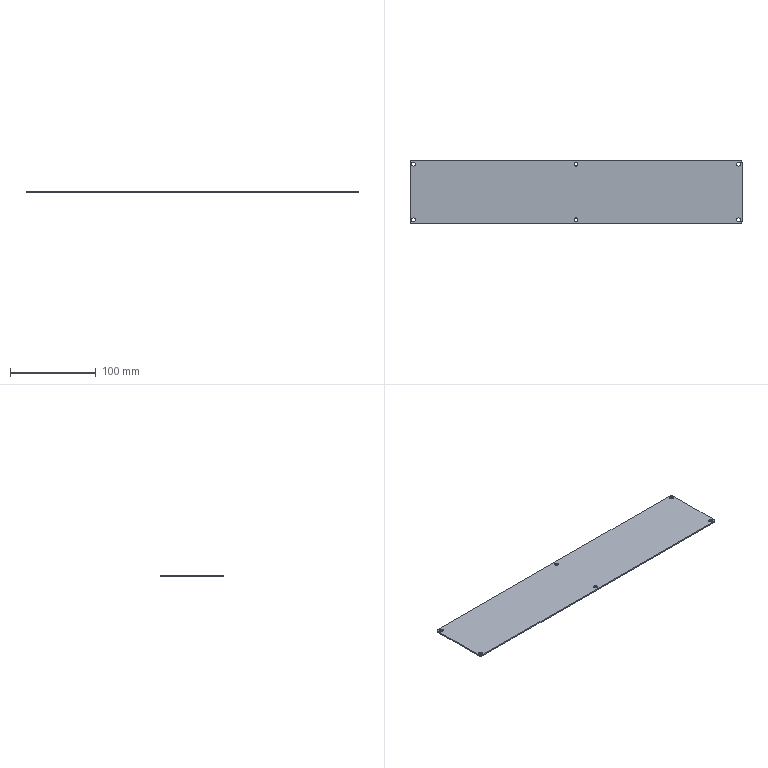Part | NX | features solid 2 | 1 solid | 22 faces | box 388 x 73 x 1.5 mm | volume 42338 mm3 | cylinder 16 | plane 6 | commonest cylinder face diameters 4.5 x12 4 x4
STEP:
#1=CARTESIAN_POINT('',(-842.,-1596.,1025.));
#2=VERTEX_POINT('',#1);
#3=CARTESIAN_POINT('',(-844.,-1598.,1025.));
#4=VERTEX_POINT('',#3);
#5=CARTESIAN_POINT('',(-842.,-1598.,1025.));
#6=DIRECTION('',(0.,0.,1.));
#7=DIRECTION('',(1.,0.,0.));
#8=AXIS2_PLACEMENT_3D('',#5,#6,#7);
#9=CIRCLE('',#8,2.);
#10=EDGE_CURVE('',#2,#4,#9,.T.);
#11=ORIENTED_EDGE('',*,*,#10,.F.);
#12=CARTESIAN_POINT('',(-842.,-1596.,1023.5));
#13=VERTEX_POINT('',#12);
#14=CARTESIAN_POINT('',(-842.,-1596.,1025.));
#15=DIRECTION('',(0.,0.,1.));
#16=VECTOR('',#15,1000.);
#17=LINE('',#14,#16);
#18=EDGE_CURVE('',#13,#2,#17,.T.);
#19=ORIENTED_EDGE('',*,*,#18,.F.);
#20=CARTESIAN_POINT('',(-844.,-1598.,1023.5));
#21=VERTEX_POINT('',#20);
#22=CARTESIAN_POINT('',(-842.,-1598.,1023.5));
#23=DIRECTION('',(0.,0.,-1.));
#24=DIRECTION('',(1.,0.,0.));
#25=AXIS2_PLACEMENT_3D('',#22,#23,#24);
#26=CIRCLE('',#25,2.);
#27=EDGE_CURVE('',#21,#13,#26,.T.);
#28=ORIENTED_EDGE('',*,*,#27,.F.);
#29=CARTESIAN_POINT('',(-844.,-1598.,1025.));
#30=DIRECTION('',(0.,0.,-1.));
#31=VECTOR('',#30,1000.);
#32=LINE('',#29,#31);
#33=EDGE_CURVE('',#4,#21,#32,.T.);
#34=ORIENTED_EDGE('',*,*,#33,.F.);
#35=EDGE_LOOP('',(#11,#19,#28,#34));
#36=FACE_BOUND('',#35,.T.);
#37=CARTESIAN_POINT('',(-842.,-1598.,1025.));
#38=DIRECTION('',(0.,0.,-1.));
#39=DIRECTION('',(-1.,0.,0.));
#40=AXIS2_PLACEMENT_3D('',#37,#38,#39);
#41=CYLINDRICAL_SURFACE('',#40,2.);
#42=ADVANCED_FACE('',(#36),#41,.T.);
#43=CARTESIAN_POINT('',(-844.,-1667.,1025.));
#44=VERTEX_POINT('',#43);
#45=CARTESIAN_POINT('',(-842.,-1669.,1025.));
#46=VERTEX_POINT('',#45);
#47=CARTESIAN_POINT('',(-842.,-1667.,1025.));
#48=DIRECTION('',(0.,0.,1.));
#49=DIRECTION('',(1.,0.,0.));
#50=AXIS2_PLACEMENT_3D('',#47,#48,#49);
#51=CIRCLE('',#50,2.);
#52=EDGE_CURVE('',#44,#46,#51,.T.);
#53=ORIENTED_EDGE('',*,*,#52,.F.);
#54=CARTESIAN_POINT('',(-844.,-1667.,1023.5));
#55=VERTEX_POINT('',#54);
#56=CARTESIAN_POINT('',(-844.,-1667.,1025.));
#57=DIRECTION('',(0.,0.,1.));
#58=VECTOR('',#57,1000.);
#59=LINE('',#56,#58);
#60=EDGE_CURVE('',#55,#44,#59,.T.);
#61=ORIENTED_EDGE('',*,*,#60,.F.);
#62=CARTESIAN_POINT('',(-842.,-1669.,1023.5));
#63=VERTEX_POINT('',#62);
#64=CARTESIAN_POINT('',(-842.,-1667.,1023.5));
#65=DIRECTION('',(0.,0.,-1.));
#66=DIRECTION('',(1.,0.,0.));
#67=AXIS2_PLACEMENT_3D('',#64,#65,#66);
#68=CIRCLE('',#67,2.);
#69=EDGE_CURVE('',#63,#55,#68,.T.);
#70=ORIENTED_EDGE('',*,*,#69,.F.);
#71=CARTESIAN_POINT('',(-842.,-1669.,1025.));
#72=DIRECTION('',(0.,0.,-1.));
#73=VECTOR('',#72,1000.);
#74=LINE('',#71,#73);
#75=EDGE_CURVE('',#46,#63,#74,.T.);
#76=ORIENTED_EDGE('',*,*,#75,.F.);
#77=EDGE_LOOP('',(#53,#61,#70,#76));
#78=FACE_BOUND('',#77,.T.);
#79=CARTESIAN_POINT('',(-842.,-1667.,1025.));
#80=DIRECTION('',(0.,0.,-1.));
#81=DIRECTION('',(-1.,0.,0.));
#82=AXIS2_PLACEMENT_3D('',#79,#80,#81);
#83=CYLINDRICAL_SURFACE('',#82,2.);
#84=ADVANCED_FACE('',(#78),#83,.T.);
#85=CARTESIAN_POINT('',(-458.,-1669.,1025.));
#86=VERTEX_POINT('',#85);
#87=CARTESIAN_POINT('',(-456.,-1667.,1025.));
#88=VERTEX_POINT('',#87);
#89=CARTESIAN_POINT('',(-458.,-1667.,1025.));
#90=DIRECTION('',(0.,0.,1.));
#91=DIRECTION('',(1.,0.,0.));
#92=AXIS2_PLACEMENT_3D('',#89,#90,#91);
#93=CIRCLE('',#92,2.);
#94=EDGE_CURVE('',#86,#88,#93,.T.);
#95=ORIENTED_EDGE('',*,*,#94,.F.);
#96=CARTESIAN_POINT('',(-458.,-1669.,1023.5));
#97=VERTEX_POINT('',#96);
#98=CARTESIAN_POINT('',(-458.,-1669.,1025.));
#99=DIRECTION('',(0.,0.,1.));
#100=VECTOR('',#99,1000.);
#101=LINE('',#98,#100);
#102=EDGE_CURVE('',#97,#86,#101,.T.);
#103=ORIENTED_EDGE('',*,*,#102,.F.);
#104=CARTESIAN_POINT('',(-456.,-1667.,1023.5));
#105=VERTEX_POINT('',#104);
#106=CARTESIAN_POINT('',(-458.,-1667.,1023.5));
#107=DIRECTION('',(0.,0.,-1.));
#108=DIRECTION('',(1.,0.,0.));
#109=AXIS2_PLACEMENT_3D('',#106,#107,#108);
#110=CIRCLE('',#109,2.);
#111=EDGE_CURVE('',#105,#97,#110,.T.);
#112=ORIENTED_EDGE('',*,*,#111,.F.);
#113=CARTESIAN_POINT('',(-456.,-1667.,1025.));
#114=DIRECTION('',(0.,0.,-1.));
#115=VECTOR('',#114,1000.);
#116=LINE('',#113,#115);
#117=EDGE_CURVE('',#88,#105,#116,.T.);
#118=ORIENTED_EDGE('',*,*,#117,.F.);
#119=EDGE_LOOP('',(#95,#103,#112,#118));
#120=FACE_BOUND('',#119,.T.);
#121=CARTESIAN_POINT('',(-458.,-1667.,1025.));
#122=DIRECTION('',(0.,0.,-1.));
#123=DIRECTION('',(-1.,0.,0.));
#124=AXIS2_PLACEMENT_3D('',#121,#122,#123);
#125=CYLINDRICAL_SURFACE('',#124,2.);
#126=ADVANCED_FACE('',(#120),#125,.T.);
#127=CARTESIAN_POINT('',(-456.,-1598.,1025.));
#128=VERTEX_POINT('',#127);
#129=CARTESIAN_POINT('',(-458.,-1596.,1025.));
#130=VERTEX_POINT('',#129);
#131=CARTESIAN_POINT('',(-458.,-1598.,1025.));
#132=DIRECTION('',(0.,0.,1.));
#133=DIRECTION('',(1.,0.,0.));
#134=AXIS2_PLACEMENT_3D('',#131,#132,#133);
#135=CIRCLE('',#134,2.);
#136=EDGE_CURVE('',#128,#130,#135,.T.);
#137=ORIENTED_EDGE('',*,*,#136,.F.);
#138=CARTESIAN_POINT('',(-456.,-1598.,1023.5));
#139=VERTEX_POINT('',#138);
#140=CARTESIAN_POINT('',(-456.,-1598.,1025.));
#141=DIRECTION('',(0.,0.,1.));
#142=VECTOR('',#141,1000.);
#143=LINE('',#140,#142);
#144=EDGE_CURVE('',#139,#128,#143,.T.);
#145=ORIENTED_EDGE('',*,*,#144,.F.);
#146=CARTESIAN_POINT('',(-458.,-1596.,1023.5));
#147=VERTEX_POINT('',#146);
#148=CARTESIAN_POINT('',(-458.,-1598.,1023.5));
#149=DIRECTION('',(0.,0.,-1.));
#150=DIRECTION('',(1.,0.,0.));
#151=AXIS2_PLACEMENT_3D('',#148,#149,#150);
#152=CIRCLE('',#151,2.);
#153=EDGE_CURVE('',#147,#139,#152,.T.);
#154=ORIENTED_EDGE('',*,*,#153,.F.);
#155=CARTESIAN_POINT('',(-458.,-1596.,1025.));
#156=DIRECTION('',(0.,0.,-1.));
#157=VECTOR('',#156,1000.);
#158=LINE('',#155,#157);
#159=EDGE_CURVE('',#130,#147,#158,.T.);
#160=ORIENTED_EDGE('',*,*,#159,.F.);
#161=EDGE_LOOP('',(#137,#145,#154,#160));
#162=FACE_BOUND('',#161,.T.);
#163=CARTESIAN_POINT('',(-458.,-1598.,1025.));
#164=DIRECTION('',(0.,0.,-1.));
#165=DIRECTION('',(-1.,0.,0.));
#166=AXIS2_PLACEMENT_3D('',#163,#164,#165);
#167=CYLINDRICAL_SURFACE('',#166,2.);
#168=ADVANCED_FACE('',(#162),#167,.T.);
#169=CARTESIAN_POINT('',(-652.25,-1600.,1025.));
#170=VERTEX_POINT('',#169);
#171=CARTESIAN_POINT('',(-652.25,-1600.,1023.5));
#172=VERTEX_POINT('',#171);
#173=CARTESIAN_POINT('',(-652.25,-1600.,630.19));
#174=DIRECTION('',(0.,0.,1.));
#175=VECTOR('',#174,1000.);
#176=LINE('',#173,#175);
#177=EDGE_CURVE('',#170,#172,#176,.F.);
#178=ORIENTED_EDGE('',*,*,#177,.T.);
#179=CARTESIAN_POINT('',(-647.75,-1600.,1023.5));
#180=VERTEX_POINT('',#179);
#181=CARTESIAN_POINT('',(-650.,-1600.,1023.5));
#182=DIRECTION('',(0.,0.,1.));
#183=DIRECTION('',(1.,0.,0.));
#184=AXIS2_PLACEMENT_3D('',#181,#182,#183);
#185=CIRCLE('',#184,2.25);
#186=EDGE_CURVE('',#180,#172,#185,.T.);
#187=ORIENTED_EDGE('',*,*,#186,.F.);
#188=CARTESIAN_POINT('',(-647.75,-1600.,1025.));
#189=VERTEX_POINT('',#188);
#190=CARTESIAN_POINT('',(-647.75,-1600.,630.19));
#191=DIRECTION('',(0.,0.,1.));
#192=VECTOR('',#191,1000.);
#193=LINE('',#190,#192);
#194=EDGE_CURVE('',#180,#189,#193,.T.);
#195=ORIENTED_EDGE('',*,*,#194,.T.);
#196=CARTESIAN_POINT('',(-650.,-1600.,1025.));
#197=DIRECTION('',(0.,0.,1.));
#198=DIRECTION('',(0.,1.,0.));
#199=AXIS2_PLACEMENT_3D('',#196,#197,#198);
#200=CIRCLE('',#199,2.25);
#201=EDGE_CURVE('',#189,#170,#200,.T.);
#202=ORIENTED_EDGE('',*,*,#201,.T.);
#203=EDGE_LOOP('',(#178,#187,#195,#202));
#204=FACE_BOUND('',#203,.T.);
#205=CARTESIAN_POINT('',(-650.,-1600.,630.19));
#206=DIRECTION('',(0.,0.,1.));
#207=DIRECTION('',(1.,0.,0.));
#208=AXIS2_PLACEMENT_3D('',#205,#206,#207);
#209=CYLINDRICAL_SURFACE('',#208,2.25);
#210=ADVANCED_FACE('',(#204),#209,.F.);
#211=CARTESIAN_POINT('',(-652.25,-1665.,1023.5));
#212=VERTEX_POINT('',#211);
#213=CARTESIAN_POINT('',(-652.25,-1665.,1025.));
#214=VERTEX_POINT('',#213);
#215=CARTESIAN_POINT('',(-652.25,-1665.,630.19));
#216=DIRECTION('',(0.,0.,1.));
#217=VECTOR('',#216,1000.);
#218=LINE('',#215,#217);
#219=EDGE_CURVE('',#212,#214,#218,.T.);
#220=ORIENTED_EDGE('',*,*,#219,.F.);
#221=CARTESIAN_POINT('',(-647.75,-1665.,1023.5));
#222=VERTEX_POINT('',#221);
#223=CARTESIAN_POINT('',(-650.,-1665.,1023.5));
#224=DIRECTION('',(0.,0.,1.));
#225=DIRECTION('',(1.,0.,0.));
#226=AXIS2_PLACEMENT_3D('',#223,#224,#225);
#227=CIRCLE('',#226,2.25);
#228=EDGE_CURVE('',#222,#212,#227,.T.);
#229=ORIENTED_EDGE('',*,*,#228,.F.);
#230=CARTESIAN_POINT('',(-647.75,-1665.,1025.));
#231=VERTEX_POINT('',#230);
#232=CARTESIAN_POINT('',(-647.75,-1665.,630.19));
#233=DIRECTION('',(0.,0.,1.));
#234=VECTOR('',#233,1000.);
#235=LINE('',#232,#234);
#236=EDGE_CURVE('',#231,#222,#235,.F.);
#237=ORIENTED_EDGE('',*,*,#236,.F.);
#238=CARTESIAN_POINT('',(-650.,-1665.,1025.));
#239=DIRECTION('',(0.,0.,1.));
#240=DIRECTION('',(0.,1.,0.));
#241=AXIS2_PLACEMENT_3D('',#238,#239,#240);
#242=CIRCLE('',#241,2.25);
#243=EDGE_CURVE('',#231,#214,#242,.T.);
#244=ORIENTED_EDGE('',*,*,#243,.T.);
#245=EDGE_LOOP('',(#220,#229,#237,#244));
#246=FACE_BOUND('',#245,.T.);
#247=CARTESIAN_POINT('',(-650.,-1665.,630.19));
#248=DIRECTION('',(0.,0.,1.));
#249=DIRECTION('',(1.,0.,0.));
#250=AXIS2_PLACEMENT_3D('',#247,#248,#249);
#251=CYLINDRICAL_SURFACE('',#250,2.25);
#252=ADVANCED_FACE('',(#246),#251,.F.);
#253=CARTESIAN_POINT('',(-842.25,-1600.,1025.));
#254=VERTEX_POINT('',#253);
#255=CARTESIAN_POINT('',(-842.25,-1600.,1023.5));
#256=VERTEX_POINT('',#255);
#257=CARTESIAN_POINT('',(-842.25,-1600.,630.19));
#258=DIRECTION('',(0.,0.,1.));
#259=VECTOR('',#258,1000.);
#260=LINE('',#257,#259);
#261=EDGE_CURVE('',#254,#256,#260,.F.);
#262=ORIENTED_EDGE('',*,*,#261,.T.);
#263=CARTESIAN_POINT('',(-837.75,-1600.,1023.5));
#264=VERTEX_POINT('',#263);
#265=CARTESIAN_POINT('',(-840.,-1600.,1023.5));
#266=DIRECTION('',(0.,0.,1.));
#267=DIRECTION('',(1.,0.,0.));
#268=AXIS2_PLACEMENT_3D('',#265,#266,#267);
#269=CIRCLE('',#268,2.25);
#270=EDGE_CURVE('',#264,#256,#269,.T.);
#271=ORIENTED_EDGE('',*,*,#270,.F.);
#272=CARTESIAN_POINT('',(-837.75,-1600.,1025.));
#273=VERTEX_POINT('',#272);
#274=CARTESIAN_POINT('',(-837.75,-1600.,630.19));
#275=DIRECTION('',(0.,0.,1.));
#276=VECTOR('',#275,1000.);
#277=LINE('',#274,#276);
#278=EDGE_CURVE('',#264,#273,#277,.T.);
#279=ORIENTED_EDGE('',*,*,#278,.T.);
#280=CARTESIAN_POINT('',(-840.,-1600.,1025.));
#281=DIRECTION('',(0.,0.,1.));
#282=DIRECTION('',(0.,1.,0.));
#283=AXIS2_PLACEMENT_3D('',#280,#281,#282);
#284=CIRCLE('',#283,2.25);
#285=EDGE_CURVE('',#273,#254,#284,.T.);
#286=ORIENTED_EDGE('',*,*,#285,.T.);
#287=EDGE_LOOP('',(#262,#271,#279,#286));
#288=FACE_BOUND('',#287,.T.);
#289=CARTESIAN_POINT('',(-840.,-1600.,630.19));
#290=DIRECTION('',(0.,0.,1.));
#291=DIRECTION('',(1.,0.,0.));
#292=AXIS2_PLACEMENT_3D('',#289,#290,#291);
#293=CYLINDRICAL_SURFACE('',#292,2.25);
#294=ADVANCED_FACE('',(#288),#293,.F.);
#295=CARTESIAN_POINT('',(-462.25,-1600.,1025.));
#296=VERTEX_POINT('',#295);
#297=CARTESIAN_POINT('',(-462.25,-1600.,1023.5));
#298=VERTEX_POINT('',#297);
#299=CARTESIAN_POINT('',(-462.25,-1600.,630.19));
#300=DIRECTION('',(0.,0.,1.));
#301=VECTOR('',#300,1000.);
#302=LINE('',#299,#301);
#303=EDGE_CURVE('',#296,#298,#302,.F.);
#304=ORIENTED_EDGE('',*,*,#303,.T.);
#305=CARTESIAN_POINT('',(-457.75,-1600.,1023.5));
#306=VERTEX_POINT('',#305);
#307=CARTESIAN_POINT('',(-460.,-1600.,1023.5));
#308=DIRECTION('',(0.,0.,1.));
#309=DIRECTION('',(1.,0.,0.));
#310=AXIS2_PLACEMENT_3D('',#307,#308,#309);
#311=CIRCLE('',#310,2.25);
#312=EDGE_CURVE('',#306,#298,#311,.T.);
#313=ORIENTED_EDGE('',*,*,#312,.F.);
#314=CARTESIAN_POINT('',(-457.75,-1600.,1025.));
#315=VERTEX_POINT('',#314);
#316=CARTESIAN_POINT('',(-457.75,-1600.,630.19));
#317=DIRECTION('',(0.,0.,1.));
#318=VECTOR('',#317,1000.);
#319=LINE('',#316,#318);
#320=EDGE_CURVE('',#306,#315,#319,.T.);
#321=ORIENTED_EDGE('',*,*,#320,.T.);
#322=CARTESIAN_POINT('',(-460.,-1600.,1025.));
#323=DIRECTION('',(0.,0.,1.));
#324=DIRECTION('',(0.,1.,0.));
#325=AXIS2_PLACEMENT_3D('',#322,#323,#324);
#326=CIRCLE('',#325,2.25);
#327=EDGE_CURVE('',#315,#296,#326,.T.);
#328=ORIENTED_EDGE('',*,*,#327,.T.);
#329=EDGE_LOOP('',(#304,#313,#321,#328));
#330=FACE_BOUND('',#329,.T.);
#331=CARTESIAN_POINT('',(-460.,-1600.,630.19));
#332=DIRECTION('',(0.,0.,1.));
#333=DIRECTION('',(1.,0.,0.));
#334=AXIS2_PLACEMENT_3D('',#331,#332,#333);
#335=CYLINDRICAL_SURFACE('',#334,2.25);
#336=ADVANCED_FACE('',(#330),#335,.F.);
#337=CARTESIAN_POINT('',(-462.25,-1665.,1023.5));
#338=VERTEX_POINT('',#337);
#339=CARTESIAN_POINT('',(-462.25,-1665.,1025.));
#340=VERTEX_POINT('',#339);
#341=CARTESIAN_POINT('',(-462.25,-1665.,630.19));
#342=DIRECTION('',(0.,0.,1.));
#343=VECTOR('',#342,1000.);
#344=LINE('',#341,#343);
#345=EDGE_CURVE('',#338,#340,#344,.T.);
#346=ORIENTED_EDGE('',*,*,#345,.F.);
#347=CARTESIAN_POINT('',(-457.75,-1665.,1023.5));
#348=VERTEX_POINT('',#347);
#349=CARTESIAN_POINT('',(-460.,-1665.,1023.5));
#350=DIRECTION('',(0.,0.,1.));
#351=DIRECTION('',(1.,0.,0.));
#352=AXIS2_PLACEMENT_3D('',#349,#350,#351);
#353=CIRCLE('',#352,2.25);
#354=EDGE_CURVE('',#348,#338,#353,.T.);
#355=ORIENTED_EDGE('',*,*,#354,.F.);
#356=CARTESIAN_POINT('',(-457.75,-1665.,1025.));
#357=VERTEX_POINT('',#356);
#358=CARTESIAN_POINT('',(-457.75,-1665.,630.19));
#359=DIRECTION('',(0.,0.,1.));
#360=VECTOR('',#359,1000.);
#361=LINE('',#358,#360);
#362=EDGE_CURVE('',#357,#348,#361,.F.);
#363=ORIENTED_EDGE('',*,*,#362,.F.);
#364=CARTESIAN_POINT('',(-460.,-1665.,1025.));
#365=DIRECTION('',(0.,0.,1.));
#366=DIRECTION('',(0.,1.,0.));
#367=AXIS2_PLACEMENT_3D('',#364,#365,#366);
#368=CIRCLE('',#367,2.25);
#369=EDGE_CURVE('',#357,#340,#368,.T.);
#370=ORIENTED_EDGE('',*,*,#369,.T.);
#371=EDGE_LOOP('',(#346,#355,#363,#370));
#372=FACE_BOUND('',#371,.T.);
#373=CARTESIAN_POINT('',(-460.,-1665.,630.19));
#374=DIRECTION('',(0.,0.,1.));
#375=DIRECTION('',(1.,0.,0.));
#376=AXIS2_PLACEMENT_3D('',#373,#374,#375);
#377=CYLINDRICAL_SURFACE('',#376,2.25);
#378=ADVANCED_FACE('',(#372),#377,.F.);
#379=CARTESIAN_POINT('',(-842.25,-1665.,1025.));
#380=VERTEX_POINT('',#379);
#381=CARTESIAN_POINT('',(-842.25,-1665.,1023.5));
#382=VERTEX_POINT('',#381);
#383=CARTESIAN_POINT('',(-842.25,-1665.,630.19));
#384=DIRECTION('',(0.,0.,1.));
#385=VECTOR('',#384,1000.);
#386=LINE('',#383,#385);
#387=EDGE_CURVE('',#380,#382,#386,.F.);
#388=ORIENTED_EDGE('',*,*,#387,.T.);
#389=CARTESIAN_POINT('',(-837.75,-1665.,1023.5));
#390=VERTEX_POINT('',#389);
#391=CARTESIAN_POINT('',(-840.,-1665.,1023.5));
#392=DIRECTION('',(0.,0.,1.));
#393=DIRECTION('',(1.,0.,0.));
#394=AXIS2_PLACEMENT_3D('',#391,#392,#393);
#395=CIRCLE('',#394,2.25);
#396=EDGE_CURVE('',#390,#382,#395,.T.);
#397=ORIENTED_EDGE('',*,*,#396,.F.);
#398=CARTESIAN_POINT('',(-837.75,-1665.,1025.));
#399=VERTEX_POINT('',#398);
#400=CARTESIAN_POINT('',(-837.75,-1665.,630.19));
#401=DIRECTION('',(0.,0.,1.));
#402=VECTOR('',#401,1000.);
#403=LINE('',#400,#402);
#404=EDGE_CURVE('',#390,#399,#403,.T.);
#405=ORIENTED_EDGE('',*,*,#404,.T.);
#406=CARTESIAN_POINT('',(-840.,-1665.,1025.));
#407=DIRECTION('',(0.,0.,1.));
#408=DIRECTION('',(0.,1.,0.));
#409=AXIS2_PLACEMENT_3D('',#406,#407,#408);
#410=CIRCLE('',#409,2.25);
#411=EDGE_CURVE('',#399,#380,#410,.T.);
#412=ORIENTED_EDGE('',*,*,#411,.T.);
#413=EDGE_LOOP('',(#388,#397,#405,#412));
#414=FACE_BOUND('',#413,.T.);
#415=CARTESIAN_POINT('',(-840.,-1665.,630.19));
#416=DIRECTION('',(0.,0.,1.));
#417=DIRECTION('',(1.,0.,0.));
#418=AXIS2_PLACEMENT_3D('',#415,#416,#417);
#419=CYLINDRICAL_SURFACE('',#418,2.25);
#420=ADVANCED_FACE('',(#414),#419,.F.);
#421=ORIENTED_EDGE('',*,*,#396,.T.);
#422=CARTESIAN_POINT('',(-840.,-1665.,1023.5));
#423=DIRECTION('',(0.,0.,1.));
#424=DIRECTION('',(1.,0.,0.));
#425=AXIS2_PLACEMENT_3D('',#422,#423,#424);
#426=CIRCLE('',#425,2.25);
#427=EDGE_CURVE('',#382,#390,#426,.T.);
#428=ORIENTED_EDGE('',*,*,#427,.T.);
#429=EDGE_LOOP('',(#421,#428));
#430=FACE_BOUND('',#429,.T.);
#431=ORIENTED_EDGE('',*,*,#354,.T.);
#432=CARTESIAN_POINT('',(-460.,-1665.,1023.5));
#433=DIRECTION('',(0.,0.,1.));
#434=DIRECTION('',(1.,0.,0.));
#435=AXIS2_PLACEMENT_3D('',#432,#433,#434);
#436=CIRCLE('',#435,2.25);
#437=EDGE_CURVE('',#338,#348,#436,.T.);
#438=ORIENTED_EDGE('',*,*,#437,.T.);
#439=EDGE_LOOP('',(#431,#438));
#440=FACE_BOUND('',#439,.T.);
#441=ORIENTED_EDGE('',*,*,#312,.T.);
#442=CARTESIAN_POINT('',(-460.,-1600.,1023.5));
#443=DIRECTION('',(0.,0.,1.));
#444=DIRECTION('',(1.,0.,0.));
#445=AXIS2_PLACEMENT_3D('',#442,#443,#444);
#446=CIRCLE('',#445,2.25);
#447=EDGE_CURVE('',#298,#306,#446,.T.);
#448=ORIENTED_EDGE('',*,*,#447,.T.);
#449=EDGE_LOOP('',(#441,#448));
#450=FACE_BOUND('',#449,.T.);
#451=ORIENTED_EDGE('',*,*,#270,.T.);
#452=CARTESIAN_POINT('',(-840.,-1600.,1023.5));
#453=DIRECTION('',(0.,0.,1.));
#454=DIRECTION('',(1.,0.,0.));
#455=AXIS2_PLACEMENT_3D('',#452,#453,#454);
#456=CIRCLE('',#455,2.25);
#457=EDGE_CURVE('',#256,#264,#456,.T.);
#458=ORIENTED_EDGE('',*,*,#457,.T.);
#459=EDGE_LOOP('',(#451,#458));
#460=FACE_BOUND('',#459,.T.);
#461=ORIENTED_EDGE('',*,*,#228,.T.);
#462=CARTESIAN_POINT('',(-650.,-1665.,1023.5));
#463=DIRECTION('',(0.,0.,1.));
#464=DIRECTION('',(1.,0.,0.));
#465=AXIS2_PLACEMENT_3D('',#462,#463,#464);
#466=CIRCLE('',#465,2.25);
#467=EDGE_CURVE('',#212,#222,#466,.T.);
#468=ORIENTED_EDGE('',*,*,#467,.T.);
#469=EDGE_LOOP('',(#461,#468));
#470=FACE_BOUND('',#469,.T.);
#471=ORIENTED_EDGE('',*,*,#186,.T.);
#472=CARTESIAN_POINT('',(-650.,-1600.,1023.5));
#473=DIRECTION('',(0.,0.,1.));
#474=DIRECTION('',(1.,0.,0.));
#475=AXIS2_PLACEMENT_3D('',#472,#473,#474);
#476=CIRCLE('',#475,2.25);
#477=EDGE_CURVE('',#172,#180,#476,.T.);
#478=ORIENTED_EDGE('',*,*,#477,.T.);
#479=EDGE_LOOP('',(#471,#478));
#480=FACE_BOUND('',#479,.T.);
#481=CARTESIAN_POINT('',(-456.,-1596.,1023.5));
#482=DIRECTION('',(-1.,0.,0.));
#483=VECTOR('',#482,1000.);
#484=LINE('',#481,#483);
#485=EDGE_CURVE('',#147,#13,#484,.T.);
#486=ORIENTED_EDGE('',*,*,#485,.F.);
#487=ORIENTED_EDGE('',*,*,#153,.T.);
#488=CARTESIAN_POINT('',(-456.,-1669.,1023.5));
#489=DIRECTION('',(0.,1.,0.));
#490=VECTOR('',#489,1000.);
#491=LINE('',#488,#490);
#492=EDGE_CURVE('',#105,#139,#491,.T.);
#493=ORIENTED_EDGE('',*,*,#492,.F.);
#494=ORIENTED_EDGE('',*,*,#111,.T.);
#495=CARTESIAN_POINT('',(-844.,-1669.,1023.5));
#496=DIRECTION('',(1.,0.,0.));
#497=VECTOR('',#496,1000.);
#498=LINE('',#495,#497);
#499=EDGE_CURVE('',#63,#97,#498,.T.);
#500=ORIENTED_EDGE('',*,*,#499,.F.);
#501=ORIENTED_EDGE('',*,*,#69,.T.);
#502=CARTESIAN_POINT('',(-844.,-1596.,1023.5));
#503=DIRECTION('',(0.,-1.,0.));
#504=VECTOR('',#503,1000.);
#505=LINE('',#502,#504);
#506=EDGE_CURVE('',#21,#55,#505,.T.);
#507=ORIENTED_EDGE('',*,*,#506,.F.);
#508=ORIENTED_EDGE('',*,*,#27,.T.);
#509=EDGE_LOOP('',(#486,#487,#493,#494,#500,#501,#507,#508));
#510=FACE_BOUND('',#509,.T.);
#511=CARTESIAN_POINT('',(-844.,-1669.,1023.5));
#512=DIRECTION('',(0.,0.,1.));
#513=DIRECTION('',(1.,0.,0.));
#514=AXIS2_PLACEMENT_3D('',#511,#512,#513);
#515=PLANE('',#514);
#516=ADVANCED_FACE('',(#430,#440,#450,#460,#470,#480,#510),#515,.F.);
#517=ORIENTED_EDGE('',*,*,#411,.F.);
#518=CARTESIAN_POINT('',(-840.,-1665.,1025.));
#519=DIRECTION('',(0.,0.,1.));
#520=DIRECTION('',(0.,1.,0.));
#521=AXIS2_PLACEMENT_3D('',#518,#519,#520);
#522=CIRCLE('',#521,2.25);
#523=EDGE_CURVE('',#380,#399,#522,.T.);
#524=ORIENTED_EDGE('',*,*,#523,.F.);
#525=EDGE_LOOP('',(#517,#524));
#526=FACE_BOUND('',#525,.T.);
#527=ORIENTED_EDGE('',*,*,#369,.F.);
#528=CARTESIAN_POINT('',(-460.,-1665.,1025.));
#529=DIRECTION('',(0.,0.,1.));
#530=DIRECTION('',(0.,1.,0.));
#531=AXIS2_PLACEMENT_3D('',#528,#529,#530);
#532=CIRCLE('',#531,2.25);
#533=EDGE_CURVE('',#340,#357,#532,.T.);
#534=ORIENTED_EDGE('',*,*,#533,.F.);
#535=EDGE_LOOP('',(#527,#534));
#536=FACE_BOUND('',#535,.T.);
#537=ORIENTED_EDGE('',*,*,#327,.F.);
#538=CARTESIAN_POINT('',(-460.,-1600.,1025.));
#539=DIRECTION('',(0.,0.,1.));
#540=DIRECTION('',(0.,1.,0.));
#541=AXIS2_PLACEMENT_3D('',#538,#539,#540);
#542=CIRCLE('',#541,2.25);
#543=EDGE_CURVE('',#296,#315,#542,.T.);
#544=ORIENTED_EDGE('',*,*,#543,.F.);
#545=EDGE_LOOP('',(#537,#544));
#546=FACE_BOUND('',#545,.T.);
#547=ORIENTED_EDGE('',*,*,#285,.F.);
#548=CARTESIAN_POINT('',(-840.,-1600.,1025.));
#549=DIRECTION('',(0.,0.,1.));
#550=DIRECTION('',(0.,1.,0.));
#551=AXIS2_PLACEMENT_3D('',#548,#549,#550);
#552=CIRCLE('',#551,2.25);
#553=EDGE_CURVE('',#254,#273,#552,.T.);
#554=ORIENTED_EDGE('',*,*,#553,.F.);
#555=EDGE_LOOP('',(#547,#554));
#556=FACE_BOUND('',#555,.T.);
#557=ORIENTED_EDGE('',*,*,#243,.F.);
#558=CARTESIAN_POINT('',(-650.,-1665.,1025.));
#559=DIRECTION('',(0.,0.,1.));
#560=DIRECTION('',(0.,1.,0.));
#561=AXIS2_PLACEMENT_3D('',#558,#559,#560);
#562=CIRCLE('',#561,2.25);
#563=EDGE_CURVE('',#214,#231,#562,.T.);
#564=ORIENTED_EDGE('',*,*,#563,.F.);
#565=EDGE_LOOP('',(#557,#564));
#566=FACE_BOUND('',#565,.T.);
#567=ORIENTED_EDGE('',*,*,#201,.F.);
#568=CARTESIAN_POINT('',(-650.,-1600.,1025.));
#569=DIRECTION('',(0.,0.,1.));
#570=DIRECTION('',(0.,1.,0.));
#571=AXIS2_PLACEMENT_3D('',#568,#569,#570);
#572=CIRCLE('',#571,2.25);
#573=EDGE_CURVE('',#170,#189,#572,.T.);
#574=ORIENTED_EDGE('',*,*,#573,.F.);
#575=EDGE_LOOP('',(#567,#574));
#576=FACE_BOUND('',#575,.T.);
#577=CARTESIAN_POINT('',(-456.,-1669.,1025.));
#578=DIRECTION('',(0.,1.,0.));
#579=VECTOR('',#578,1000.);
#580=LINE('',#577,#579);
#581=EDGE_CURVE('',#88,#128,#580,.T.);
#582=ORIENTED_EDGE('',*,*,#581,.T.);
#583=ORIENTED_EDGE('',*,*,#136,.T.);
#584=CARTESIAN_POINT('',(-456.,-1596.,1025.));
#585=DIRECTION('',(-1.,0.,0.));
#586=VECTOR('',#585,1000.);
#587=LINE('',#584,#586);
#588=EDGE_CURVE('',#130,#2,#587,.T.);
#589=ORIENTED_EDGE('',*,*,#588,.T.);
#590=ORIENTED_EDGE('',*,*,#10,.T.);
#591=CARTESIAN_POINT('',(-844.,-1596.,1025.));
#592=DIRECTION('',(0.,-1.,0.));
#593=VECTOR('',#592,1000.);
#594=LINE('',#591,#593);
#595=EDGE_CURVE('',#4,#44,#594,.T.);
#596=ORIENTED_EDGE('',*,*,#595,.T.);
#597=ORIENTED_EDGE('',*,*,#52,.T.);
#598=CARTESIAN_POINT('',(-844.,-1669.,1025.));
#599=DIRECTION('',(1.,0.,0.));
#600=VECTOR('',#599,1000.);
#601=LINE('',#598,#600);
#602=EDGE_CURVE('',#46,#86,#601,.T.);
#603=ORIENTED_EDGE('',*,*,#602,.T.);
#604=ORIENTED_EDGE('',*,*,#94,.T.);
#605=EDGE_LOOP('',(#582,#583,#589,#590,#596,#597,#603,#604));
#606=FACE_BOUND('',#605,.T.);
#607=CARTESIAN_POINT('',(-844.,-1669.,1025.));
#608=DIRECTION('',(0.,0.,1.));
#609=DIRECTION('',(1.,0.,0.));
#610=AXIS2_PLACEMENT_3D('',#607,#608,#609);
#611=PLANE('',#610);
#612=ADVANCED_FACE('',(#526,#536,#546,#556,#566,#576,#606),#611,.T.);
#613=ORIENTED_EDGE('',*,*,#588,.F.);
#614=ORIENTED_EDGE('',*,*,#159,.T.);
#615=ORIENTED_EDGE('',*,*,#485,.T.);
#616=ORIENTED_EDGE('',*,*,#18,.T.);
#617=EDGE_LOOP('',(#613,#614,#615,#616));
#618=FACE_BOUND('',#617,.T.);
#619=CARTESIAN_POINT('',(-456.,-1596.,1025.));
#620=DIRECTION('',(0.,-1.,0.));
#621=DIRECTION('',(0.,0.,-1.));
#622=AXIS2_PLACEMENT_3D('',#619,#620,#621);
#623=PLANE('',#622);
#624=ADVANCED_FACE('',(#618),#623,.F.);
#625=ORIENTED_EDGE('',*,*,#492,.T.);
#626=ORIENTED_EDGE('',*,*,#144,.T.);
#627=ORIENTED_EDGE('',*,*,#581,.F.);
#628=ORIENTED_EDGE('',*,*,#117,.T.);
#629=EDGE_LOOP('',(#625,#626,#627,#628));
#630=FACE_BOUND('',#629,.T.);
#631=CARTESIAN_POINT('',(-456.,-1669.,1025.));
#632=DIRECTION('',(-1.,0.,0.));
#633=DIRECTION('',(0.,0.,1.));
#634=AXIS2_PLACEMENT_3D('',#631,#632,#633);
#635=PLANE('',#634);
#636=ADVANCED_FACE('',(#630),#635,.F.);
#637=ORIENTED_EDGE('',*,*,#499,.T.);
#638=ORIENTED_EDGE('',*,*,#102,.T.);
#639=ORIENTED_EDGE('',*,*,#602,.F.);
#640=ORIENTED_EDGE('',*,*,#75,.T.);
#641=EDGE_LOOP('',(#637,#638,#639,#640));
#642=FACE_BOUND('',#641,.T.);
#643=CARTESIAN_POINT('',(-844.,-1669.,1025.));
#644=DIRECTION('',(0.,1.,0.));
#645=DIRECTION('',(1.,0.,0.));
#646=AXIS2_PLACEMENT_3D('',#643,#644,#645);
#647=PLANE('',#646);
#648=ADVANCED_FACE('',(#642),#647,.F.);
#649=ORIENTED_EDGE('',*,*,#506,.T.);
#650=ORIENTED_EDGE('',*,*,#60,.T.);
#651=ORIENTED_EDGE('',*,*,#595,.F.);
#652=ORIENTED_EDGE('',*,*,#33,.T.);
#653=EDGE_LOOP('',(#649,#650,#651,#652));
#654=FACE_BOUND('',#653,.T.);
#655=CARTESIAN_POINT('',(-844.,-1596.,1025.));
#656=DIRECTION('',(1.,0.,0.));
#657=DIRECTION('',(0.,1.,0.));
#658=AXIS2_PLACEMENT_3D('',#655,#656,#657);
#659=PLANE('',#658);
#660=ADVANCED_FACE('',(#654),#659,.F.);
#661=ORIENTED_EDGE('',*,*,#427,.F.);
#662=ORIENTED_EDGE('',*,*,#387,.F.);
#663=ORIENTED_EDGE('',*,*,#523,.T.);
#664=ORIENTED_EDGE('',*,*,#404,.F.);
#665=EDGE_LOOP('',(#661,#662,#663,#664));
#666=FACE_BOUND('',#665,.T.);
#667=CARTESIAN_POINT('',(-840.,-1665.,630.19));
#668=DIRECTION('',(0.,0.,1.));
#669=DIRECTION('',(1.,0.,0.));
#670=AXIS2_PLACEMENT_3D('',#667,#668,#669);
#671=CYLINDRICAL_SURFACE('',#670,2.25);
#672=ADVANCED_FACE('',(#666),#671,.F.);
#673=ORIENTED_EDGE('',*,*,#437,.F.);
#674=ORIENTED_EDGE('',*,*,#345,.T.);
#675=ORIENTED_EDGE('',*,*,#533,.T.);
#676=ORIENTED_EDGE('',*,*,#362,.T.);
#677=EDGE_LOOP('',(#673,#674,#675,#676));
#678=FACE_BOUND('',#677,.T.);
#679=CARTESIAN_POINT('',(-460.,-1665.,630.19));
#680=DIRECTION('',(0.,0.,1.));
#681=DIRECTION('',(1.,0.,0.));
#682=AXIS2_PLACEMENT_3D('',#679,#680,#681);
#683=CYLINDRICAL_SURFACE('',#682,2.25);
#684=ADVANCED_FACE('',(#678),#683,.F.);
#685=ORIENTED_EDGE('',*,*,#447,.F.);
#686=ORIENTED_EDGE('',*,*,#303,.F.);
#687=ORIENTED_EDGE('',*,*,#543,.T.);
#688=ORIENTED_EDGE('',*,*,#320,.F.);
#689=EDGE_LOOP('',(#685,#686,#687,#688));
#690=FACE_BOUND('',#689,.T.);
#691=CARTESIAN_POINT('',(-460.,-1600.,630.19));
#692=DIRECTION('',(0.,0.,1.));
#693=DIRECTION('',(1.,0.,0.));
#694=AXIS2_PLACEMENT_3D('',#691,#692,#693);
#695=CYLINDRICAL_SURFACE('',#694,2.25);
#696=ADVANCED_FACE('',(#690),#695,.F.);
#697=ORIENTED_EDGE('',*,*,#457,.F.);
#698=ORIENTED_EDGE('',*,*,#261,.F.);
#699=ORIENTED_EDGE('',*,*,#553,.T.);
#700=ORIENTED_EDGE('',*,*,#278,.F.);
#701=EDGE_LOOP('',(#697,#698,#699,#700));
#702=FACE_BOUND('',#701,.T.);
#703=CARTESIAN_POINT('',(-840.,-1600.,630.19));
#704=DIRECTION('',(0.,0.,1.));
#705=DIRECTION('',(1.,0.,0.));
#706=AXIS2_PLACEMENT_3D('',#703,#704,#705);
#707=CYLINDRICAL_SURFACE('',#706,2.25);
#708=ADVANCED_FACE('',(#702),#707,.F.);
#709=ORIENTED_EDGE('',*,*,#467,.F.);
#710=ORIENTED_EDGE('',*,*,#219,.T.);
#711=ORIENTED_EDGE('',*,*,#563,.T.);
#712=ORIENTED_EDGE('',*,*,#236,.T.);
#713=EDGE_LOOP('',(#709,#710,#711,#712));
#714=FACE_BOUND('',#713,.T.);
#715=CARTESIAN_POINT('',(-650.,-1665.,630.19));
#716=DIRECTION('',(0.,0.,1.));
#717=DIRECTION('',(1.,0.,0.));
#718=AXIS2_PLACEMENT_3D('',#715,#716,#717);
#719=CYLINDRICAL_SURFACE('',#718,2.25);
#720=ADVANCED_FACE('',(#714),#719,.F.);
#721=ORIENTED_EDGE('',*,*,#477,.F.);
#722=ORIENTED_EDGE('',*,*,#177,.F.);
#723=ORIENTED_EDGE('',*,*,#573,.T.);
#724=ORIENTED_EDGE('',*,*,#194,.F.);
#725=EDGE_LOOP('',(#721,#722,#723,#724));
#726=FACE_BOUND('',#725,.T.);
#727=CARTESIAN_POINT('',(-650.,-1600.,630.19));
#728=DIRECTION('',(0.,0.,1.));
#729=DIRECTION('',(1.,0.,0.));
#730=AXIS2_PLACEMENT_3D('',#727,#728,#729);
#731=CYLINDRICAL_SURFACE('',#730,2.25);
#732=ADVANCED_FACE('',(#726),#731,.F.);
#733=CLOSED_SHELL('',(#42,#84,#126,#168,#210,#252,#294,#336,#378,#420,#516,#612,#624,#636,#648,#660,#672,#684,#696,#708,#720,#732));
#734=MANIFOLD_SOLID_BREP('',#733);
#735=(LENGTH_UNIT()NAMED_UNIT(*)SI_UNIT(.MILLI.,.METRE.));
#736=UNCERTAINTY_MEASURE_WITH_UNIT(LENGTH_MEASURE(0.00001),#735,'','');
#737=(NAMED_UNIT(*)PLANE_ANGLE_UNIT()SI_UNIT($,.RADIAN.));
#738=(NAMED_UNIT(*)SI_UNIT($,.STERADIAN.)SOLID_ANGLE_UNIT());
#739=(GEOMETRIC_REPRESENTATION_CONTEXT(3)GLOBAL_UNCERTAINTY_ASSIGNED_CONTEXT((#736))GLOBAL_UNIT_ASSIGNED_CONTEXT((#735,#737,#738))REPRESENTATION_CONTEXT('',''));
#740=ADVANCED_BREP_SHAPE_REPRESENTATION('',(#734),#739);